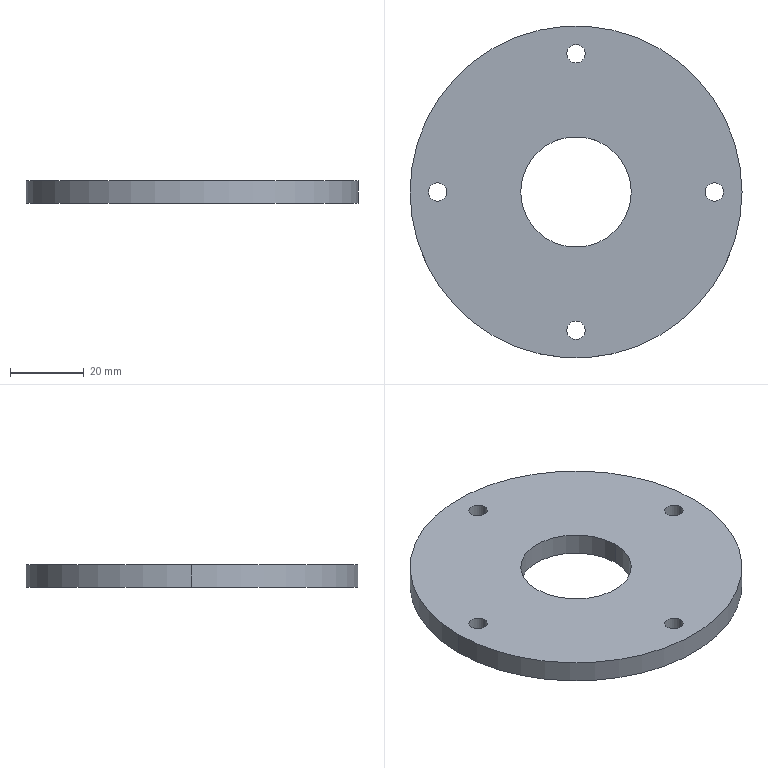Part | SolidWorks | features FlatPattern 1, HoleWzd 1, SMBaseFlange 1, SheetMetal 1 | 1 solid | 14 faces | box 90 x 90 x 6 mm | volume 33458 mm3 | cylinder 12 | plane 2 | commonest cylinder face diameters 5 x8 30 x2 90 x2
STEP:
#1=CARTESIAN_POINT('',(-2.5,37.5,-6.));
#2=VERTEX_POINT('',#1);
#3=CARTESIAN_POINT('',(2.5,37.5,-6.));
#4=VERTEX_POINT('',#3);
#5=CARTESIAN_POINT('',(0.,37.5,-6.));
#6=DIRECTION('',(0.,0.,1.));
#7=DIRECTION('',(1.,0.,0.));
#8=AXIS2_PLACEMENT_3D('',#5,#6,#7);
#9=CIRCLE('',#8,2.5);
#10=EDGE_CURVE('',#2,#4,#9,.T.);
#11=ORIENTED_EDGE('',*,*,#10,.F.);
#12=CARTESIAN_POINT('',(-2.5,37.5,0.));
#13=VERTEX_POINT('',#12);
#14=CARTESIAN_POINT('',(-2.5,37.5,0.));
#15=DIRECTION('',(0.,0.,1.));
#16=VECTOR('',#15,1000.);
#17=LINE('',#14,#16);
#18=EDGE_CURVE('',#2,#13,#17,.T.);
#19=ORIENTED_EDGE('',*,*,#18,.T.);
#20=CARTESIAN_POINT('',(2.5,37.5,0.));
#21=VERTEX_POINT('',#20);
#22=CARTESIAN_POINT('',(0.,37.5,0.));
#23=DIRECTION('',(0.,0.,1.));
#24=DIRECTION('',(1.,0.,0.));
#25=AXIS2_PLACEMENT_3D('',#22,#23,#24);
#26=CIRCLE('',#25,2.5);
#27=EDGE_CURVE('',#13,#21,#26,.T.);
#28=ORIENTED_EDGE('',*,*,#27,.T.);
#29=CARTESIAN_POINT('',(2.5,37.5,0.));
#30=DIRECTION('',(0.,0.,1.));
#31=VECTOR('',#30,1000.);
#32=LINE('',#29,#31);
#33=EDGE_CURVE('',#4,#21,#32,.T.);
#34=ORIENTED_EDGE('',*,*,#33,.F.);
#35=EDGE_LOOP('',(#11,#19,#28,#34));
#36=FACE_OUTER_BOUND('',#35,.T.);
#37=CARTESIAN_POINT('',(0.,37.5,0.));
#38=DIRECTION('',(0.,0.,1.));
#39=DIRECTION('',(1.,0.,0.));
#40=AXIS2_PLACEMENT_3D('',#37,#38,#39);
#41=CYLINDRICAL_SURFACE('',#40,2.5);
#42=ADVANCED_FACE('',(#36),#41,.F.);
#43=CARTESIAN_POINT('',(35.,0.,-6.));
#44=VERTEX_POINT('',#43);
#45=CARTESIAN_POINT('',(40.,0.,-6.));
#46=VERTEX_POINT('',#45);
#47=CARTESIAN_POINT('',(37.5,0.,-6.));
#48=DIRECTION('',(0.,0.,1.));
#49=DIRECTION('',(1.,0.,0.));
#50=AXIS2_PLACEMENT_3D('',#47,#48,#49);
#51=CIRCLE('',#50,2.5);
#52=EDGE_CURVE('',#44,#46,#51,.T.);
#53=ORIENTED_EDGE('',*,*,#52,.F.);
#54=CARTESIAN_POINT('',(35.,0.,0.));
#55=VERTEX_POINT('',#54);
#56=CARTESIAN_POINT('',(35.,0.,0.));
#57=DIRECTION('',(0.,0.,1.));
#58=VECTOR('',#57,1000.);
#59=LINE('',#56,#58);
#60=EDGE_CURVE('',#44,#55,#59,.T.);
#61=ORIENTED_EDGE('',*,*,#60,.T.);
#62=CARTESIAN_POINT('',(40.,0.,0.));
#63=VERTEX_POINT('',#62);
#64=CARTESIAN_POINT('',(37.5,0.,0.));
#65=DIRECTION('',(0.,0.,1.));
#66=DIRECTION('',(1.,0.,0.));
#67=AXIS2_PLACEMENT_3D('',#64,#65,#66);
#68=CIRCLE('',#67,2.5);
#69=EDGE_CURVE('',#55,#63,#68,.T.);
#70=ORIENTED_EDGE('',*,*,#69,.T.);
#71=CARTESIAN_POINT('',(40.,0.,0.));
#72=DIRECTION('',(0.,0.,1.));
#73=VECTOR('',#72,1000.);
#74=LINE('',#71,#73);
#75=EDGE_CURVE('',#46,#63,#74,.T.);
#76=ORIENTED_EDGE('',*,*,#75,.F.);
#77=EDGE_LOOP('',(#53,#61,#70,#76));
#78=FACE_OUTER_BOUND('',#77,.T.);
#79=CARTESIAN_POINT('',(37.5,0.,0.));
#80=DIRECTION('',(0.,0.,1.));
#81=DIRECTION('',(1.,0.,0.));
#82=AXIS2_PLACEMENT_3D('',#79,#80,#81);
#83=CYLINDRICAL_SURFACE('',#82,2.5);
#84=ADVANCED_FACE('',(#78),#83,.F.);
#85=CARTESIAN_POINT('',(-2.5,-37.5,-6.));
#86=VERTEX_POINT('',#85);
#87=CARTESIAN_POINT('',(2.5,-37.5,-6.));
#88=VERTEX_POINT('',#87);
#89=CARTESIAN_POINT('',(0.,-37.5,-6.));
#90=DIRECTION('',(0.,0.,1.));
#91=DIRECTION('',(1.,0.,0.));
#92=AXIS2_PLACEMENT_3D('',#89,#90,#91);
#93=CIRCLE('',#92,2.5);
#94=EDGE_CURVE('',#86,#88,#93,.T.);
#95=ORIENTED_EDGE('',*,*,#94,.F.);
#96=CARTESIAN_POINT('',(-2.5,-37.5,0.));
#97=VERTEX_POINT('',#96);
#98=CARTESIAN_POINT('',(-2.5,-37.5,0.));
#99=DIRECTION('',(0.,0.,1.));
#100=VECTOR('',#99,1000.);
#101=LINE('',#98,#100);
#102=EDGE_CURVE('',#86,#97,#101,.T.);
#103=ORIENTED_EDGE('',*,*,#102,.T.);
#104=CARTESIAN_POINT('',(2.5,-37.5,0.));
#105=VERTEX_POINT('',#104);
#106=CARTESIAN_POINT('',(0.,-37.5,0.));
#107=DIRECTION('',(0.,0.,1.));
#108=DIRECTION('',(1.,0.,0.));
#109=AXIS2_PLACEMENT_3D('',#106,#107,#108);
#110=CIRCLE('',#109,2.5);
#111=EDGE_CURVE('',#97,#105,#110,.T.);
#112=ORIENTED_EDGE('',*,*,#111,.T.);
#113=CARTESIAN_POINT('',(2.5,-37.5,0.));
#114=DIRECTION('',(0.,0.,1.));
#115=VECTOR('',#114,1000.);
#116=LINE('',#113,#115);
#117=EDGE_CURVE('',#88,#105,#116,.T.);
#118=ORIENTED_EDGE('',*,*,#117,.F.);
#119=EDGE_LOOP('',(#95,#103,#112,#118));
#120=FACE_OUTER_BOUND('',#119,.T.);
#121=CARTESIAN_POINT('',(0.,-37.5,0.));
#122=DIRECTION('',(0.,0.,1.));
#123=DIRECTION('',(1.,0.,0.));
#124=AXIS2_PLACEMENT_3D('',#121,#122,#123);
#125=CYLINDRICAL_SURFACE('',#124,2.5);
#126=ADVANCED_FACE('',(#120),#125,.F.);
#127=CARTESIAN_POINT('',(-40.,0.,-6.));
#128=VERTEX_POINT('',#127);
#129=CARTESIAN_POINT('',(-35.,0.,-6.));
#130=VERTEX_POINT('',#129);
#131=CARTESIAN_POINT('',(-37.5,0.,-6.));
#132=DIRECTION('',(0.,0.,1.));
#133=DIRECTION('',(1.,0.,0.));
#134=AXIS2_PLACEMENT_3D('',#131,#132,#133);
#135=CIRCLE('',#134,2.5);
#136=EDGE_CURVE('',#128,#130,#135,.T.);
#137=ORIENTED_EDGE('',*,*,#136,.F.);
#138=CARTESIAN_POINT('',(-40.,0.,0.));
#139=VERTEX_POINT('',#138);
#140=CARTESIAN_POINT('',(-40.,0.,0.));
#141=DIRECTION('',(0.,0.,1.));
#142=VECTOR('',#141,1000.);
#143=LINE('',#140,#142);
#144=EDGE_CURVE('',#128,#139,#143,.T.);
#145=ORIENTED_EDGE('',*,*,#144,.T.);
#146=CARTESIAN_POINT('',(-35.,0.,0.));
#147=VERTEX_POINT('',#146);
#148=CARTESIAN_POINT('',(-37.5,0.,0.));
#149=DIRECTION('',(0.,0.,1.));
#150=DIRECTION('',(1.,0.,0.));
#151=AXIS2_PLACEMENT_3D('',#148,#149,#150);
#152=CIRCLE('',#151,2.5);
#153=EDGE_CURVE('',#139,#147,#152,.T.);
#154=ORIENTED_EDGE('',*,*,#153,.T.);
#155=CARTESIAN_POINT('',(-35.,0.,0.));
#156=DIRECTION('',(0.,0.,1.));
#157=VECTOR('',#156,1000.);
#158=LINE('',#155,#157);
#159=EDGE_CURVE('',#130,#147,#158,.T.);
#160=ORIENTED_EDGE('',*,*,#159,.F.);
#161=EDGE_LOOP('',(#137,#145,#154,#160));
#162=FACE_OUTER_BOUND('',#161,.T.);
#163=CARTESIAN_POINT('',(-37.5,0.,0.));
#164=DIRECTION('',(0.,0.,1.));
#165=DIRECTION('',(1.,0.,0.));
#166=AXIS2_PLACEMENT_3D('',#163,#164,#165);
#167=CYLINDRICAL_SURFACE('',#166,2.5);
#168=ADVANCED_FACE('',(#162),#167,.F.);
#169=CARTESIAN_POINT('',(-15.,0.,-6.));
#170=VERTEX_POINT('',#169);
#171=CARTESIAN_POINT('',(15.,0.,-6.));
#172=VERTEX_POINT('',#171);
#173=CARTESIAN_POINT('',(0.,0.,-6.));
#174=DIRECTION('',(0.,0.,1.));
#175=DIRECTION('',(1.,0.,0.));
#176=AXIS2_PLACEMENT_3D('',#173,#174,#175);
#177=CIRCLE('',#176,15.);
#178=EDGE_CURVE('',#170,#172,#177,.T.);
#179=ORIENTED_EDGE('',*,*,#178,.F.);
#180=CARTESIAN_POINT('',(-15.,0.,0.));
#181=VERTEX_POINT('',#180);
#182=CARTESIAN_POINT('',(-15.,0.,-6.));
#183=DIRECTION('',(0.,0.,1.));
#184=VECTOR('',#183,1000.);
#185=LINE('',#182,#184);
#186=EDGE_CURVE('',#170,#181,#185,.T.);
#187=ORIENTED_EDGE('',*,*,#186,.T.);
#188=CARTESIAN_POINT('',(15.,0.,0.));
#189=VERTEX_POINT('',#188);
#190=CARTESIAN_POINT('',(0.,0.,0.));
#191=DIRECTION('',(0.,0.,1.));
#192=DIRECTION('',(1.,0.,0.));
#193=AXIS2_PLACEMENT_3D('',#190,#191,#192);
#194=CIRCLE('',#193,15.);
#195=EDGE_CURVE('',#181,#189,#194,.T.);
#196=ORIENTED_EDGE('',*,*,#195,.T.);
#197=CARTESIAN_POINT('',(15.,0.,-6.));
#198=DIRECTION('',(0.,0.,1.));
#199=VECTOR('',#198,1000.);
#200=LINE('',#197,#199);
#201=EDGE_CURVE('',#172,#189,#200,.T.);
#202=ORIENTED_EDGE('',*,*,#201,.F.);
#203=EDGE_LOOP('',(#179,#187,#196,#202));
#204=FACE_OUTER_BOUND('',#203,.T.);
#205=CARTESIAN_POINT('',(0.,0.,-6.));
#206=DIRECTION('',(0.,0.,1.));
#207=DIRECTION('',(1.,0.,0.));
#208=AXIS2_PLACEMENT_3D('',#205,#206,#207);
#209=CYLINDRICAL_SURFACE('',#208,15.);
#210=ADVANCED_FACE('',(#204),#209,.F.);
#211=CARTESIAN_POINT('',(45.,0.,-6.));
#212=VERTEX_POINT('',#211);
#213=CARTESIAN_POINT('',(-45.,0.,-6.));
#214=VERTEX_POINT('',#213);
#215=CARTESIAN_POINT('',(0.,0.,-6.));
#216=DIRECTION('',(0.,0.,1.));
#217=DIRECTION('',(1.,0.,0.));
#218=AXIS2_PLACEMENT_3D('',#215,#216,#217);
#219=CIRCLE('',#218,45.);
#220=EDGE_CURVE('',#212,#214,#219,.T.);
#221=ORIENTED_EDGE('',*,*,#220,.T.);
#222=CARTESIAN_POINT('',(-45.,0.,0.));
#223=VERTEX_POINT('',#222);
#224=CARTESIAN_POINT('',(-45.,0.,-6.));
#225=DIRECTION('',(0.,0.,1.));
#226=VECTOR('',#225,1000.);
#227=LINE('',#224,#226);
#228=EDGE_CURVE('',#214,#223,#227,.T.);
#229=ORIENTED_EDGE('',*,*,#228,.T.);
#230=CARTESIAN_POINT('',(45.,0.,0.));
#231=VERTEX_POINT('',#230);
#232=CARTESIAN_POINT('',(0.,0.,0.));
#233=DIRECTION('',(0.,0.,1.));
#234=DIRECTION('',(1.,0.,0.));
#235=AXIS2_PLACEMENT_3D('',#232,#233,#234);
#236=CIRCLE('',#235,45.);
#237=EDGE_CURVE('',#231,#223,#236,.T.);
#238=ORIENTED_EDGE('',*,*,#237,.F.);
#239=CARTESIAN_POINT('',(45.,0.,-6.));
#240=DIRECTION('',(0.,0.,1.));
#241=VECTOR('',#240,1000.);
#242=LINE('',#239,#241);
#243=EDGE_CURVE('',#212,#231,#242,.T.);
#244=ORIENTED_EDGE('',*,*,#243,.F.);
#245=EDGE_LOOP('',(#221,#229,#238,#244));
#246=FACE_OUTER_BOUND('',#245,.T.);
#247=CARTESIAN_POINT('',(0.,0.,-6.));
#248=DIRECTION('',(0.,0.,1.));
#249=DIRECTION('',(1.,0.,0.));
#250=AXIS2_PLACEMENT_3D('',#247,#248,#249);
#251=CYLINDRICAL_SURFACE('',#250,45.);
#252=ADVANCED_FACE('',(#246),#251,.T.);
#253=ORIENTED_EDGE('',*,*,#228,.F.);
#254=CARTESIAN_POINT('',(0.,0.,-6.));
#255=DIRECTION('',(0.,0.,1.));
#256=DIRECTION('',(1.,0.,0.));
#257=AXIS2_PLACEMENT_3D('',#254,#255,#256);
#258=CIRCLE('',#257,45.);
#259=EDGE_CURVE('',#214,#212,#258,.T.);
#260=ORIENTED_EDGE('',*,*,#259,.T.);
#261=ORIENTED_EDGE('',*,*,#243,.T.);
#262=CARTESIAN_POINT('',(0.,0.,0.));
#263=DIRECTION('',(0.,0.,1.));
#264=DIRECTION('',(1.,0.,0.));
#265=AXIS2_PLACEMENT_3D('',#262,#263,#264);
#266=CIRCLE('',#265,45.);
#267=EDGE_CURVE('',#223,#231,#266,.T.);
#268=ORIENTED_EDGE('',*,*,#267,.F.);
#269=EDGE_LOOP('',(#253,#260,#261,#268));
#270=FACE_OUTER_BOUND('',#269,.T.);
#271=CARTESIAN_POINT('',(0.,0.,-6.));
#272=DIRECTION('',(0.,0.,1.));
#273=DIRECTION('',(1.,0.,0.));
#274=AXIS2_PLACEMENT_3D('',#271,#272,#273);
#275=CYLINDRICAL_SURFACE('',#274,45.);
#276=ADVANCED_FACE('',(#270),#275,.T.);
#277=CARTESIAN_POINT('',(0.,37.5,-6.));
#278=DIRECTION('',(0.,0.,1.));
#279=DIRECTION('',(1.,0.,0.));
#280=AXIS2_PLACEMENT_3D('',#277,#278,#279);
#281=CIRCLE('',#280,2.5);
#282=EDGE_CURVE('',#4,#2,#281,.T.);
#283=ORIENTED_EDGE('',*,*,#282,.T.);
#284=ORIENTED_EDGE('',*,*,#10,.T.);
#285=EDGE_LOOP('',(#283,#284));
#286=FACE_BOUND('',#285,.T.);
#287=CARTESIAN_POINT('',(37.5,0.,-6.));
#288=DIRECTION('',(0.,0.,1.));
#289=DIRECTION('',(1.,0.,0.));
#290=AXIS2_PLACEMENT_3D('',#287,#288,#289);
#291=CIRCLE('',#290,2.5);
#292=EDGE_CURVE('',#46,#44,#291,.T.);
#293=ORIENTED_EDGE('',*,*,#292,.T.);
#294=ORIENTED_EDGE('',*,*,#52,.T.);
#295=EDGE_LOOP('',(#293,#294));
#296=FACE_BOUND('',#295,.T.);
#297=CARTESIAN_POINT('',(0.,-37.5,-6.));
#298=DIRECTION('',(0.,0.,1.));
#299=DIRECTION('',(1.,0.,0.));
#300=AXIS2_PLACEMENT_3D('',#297,#298,#299);
#301=CIRCLE('',#300,2.5);
#302=EDGE_CURVE('',#88,#86,#301,.T.);
#303=ORIENTED_EDGE('',*,*,#302,.T.);
#304=ORIENTED_EDGE('',*,*,#94,.T.);
#305=EDGE_LOOP('',(#303,#304));
#306=FACE_BOUND('',#305,.T.);
#307=CARTESIAN_POINT('',(-37.5,0.,-6.));
#308=DIRECTION('',(0.,0.,1.));
#309=DIRECTION('',(1.,0.,0.));
#310=AXIS2_PLACEMENT_3D('',#307,#308,#309);
#311=CIRCLE('',#310,2.5);
#312=EDGE_CURVE('',#130,#128,#311,.T.);
#313=ORIENTED_EDGE('',*,*,#312,.T.);
#314=ORIENTED_EDGE('',*,*,#136,.T.);
#315=EDGE_LOOP('',(#313,#314));
#316=FACE_BOUND('',#315,.T.);
#317=CARTESIAN_POINT('',(0.,0.,-6.));
#318=DIRECTION('',(0.,0.,1.));
#319=DIRECTION('',(1.,0.,0.));
#320=AXIS2_PLACEMENT_3D('',#317,#318,#319);
#321=CIRCLE('',#320,15.);
#322=EDGE_CURVE('',#172,#170,#321,.T.);
#323=ORIENTED_EDGE('',*,*,#322,.T.);
#324=ORIENTED_EDGE('',*,*,#178,.T.);
#325=EDGE_LOOP('',(#323,#324));
#326=FACE_BOUND('',#325,.T.);
#327=ORIENTED_EDGE('',*,*,#220,.F.);
#328=ORIENTED_EDGE('',*,*,#259,.F.);
#329=EDGE_LOOP('',(#327,#328));
#330=FACE_OUTER_BOUND('',#329,.T.);
#331=CARTESIAN_POINT('',(0.,0.,-6.));
#332=DIRECTION('',(0.,0.,1.));
#333=DIRECTION('',(1.,0.,0.));
#334=AXIS2_PLACEMENT_3D('',#331,#332,#333);
#335=PLANE('',#334);
#336=ADVANCED_FACE('',(#286,#296,#306,#316,#326,#330),#335,.F.);
#337=CARTESIAN_POINT('',(0.,37.5,0.));
#338=DIRECTION('',(0.,0.,1.));
#339=DIRECTION('',(1.,0.,0.));
#340=AXIS2_PLACEMENT_3D('',#337,#338,#339);
#341=CIRCLE('',#340,2.5);
#342=EDGE_CURVE('',#21,#13,#341,.T.);
#343=ORIENTED_EDGE('',*,*,#342,.F.);
#344=ORIENTED_EDGE('',*,*,#27,.F.);
#345=EDGE_LOOP('',(#343,#344));
#346=FACE_BOUND('',#345,.T.);
#347=CARTESIAN_POINT('',(37.5,0.,0.));
#348=DIRECTION('',(0.,0.,1.));
#349=DIRECTION('',(1.,0.,0.));
#350=AXIS2_PLACEMENT_3D('',#347,#348,#349);
#351=CIRCLE('',#350,2.5);
#352=EDGE_CURVE('',#63,#55,#351,.T.);
#353=ORIENTED_EDGE('',*,*,#352,.F.);
#354=ORIENTED_EDGE('',*,*,#69,.F.);
#355=EDGE_LOOP('',(#353,#354));
#356=FACE_BOUND('',#355,.T.);
#357=CARTESIAN_POINT('',(0.,-37.5,0.));
#358=DIRECTION('',(0.,0.,1.));
#359=DIRECTION('',(1.,0.,0.));
#360=AXIS2_PLACEMENT_3D('',#357,#358,#359);
#361=CIRCLE('',#360,2.5);
#362=EDGE_CURVE('',#105,#97,#361,.T.);
#363=ORIENTED_EDGE('',*,*,#362,.F.);
#364=ORIENTED_EDGE('',*,*,#111,.F.);
#365=EDGE_LOOP('',(#363,#364));
#366=FACE_BOUND('',#365,.T.);
#367=CARTESIAN_POINT('',(-37.5,0.,0.));
#368=DIRECTION('',(0.,0.,1.));
#369=DIRECTION('',(1.,0.,0.));
#370=AXIS2_PLACEMENT_3D('',#367,#368,#369);
#371=CIRCLE('',#370,2.5);
#372=EDGE_CURVE('',#147,#139,#371,.T.);
#373=ORIENTED_EDGE('',*,*,#372,.F.);
#374=ORIENTED_EDGE('',*,*,#153,.F.);
#375=EDGE_LOOP('',(#373,#374));
#376=FACE_BOUND('',#375,.T.);
#377=CARTESIAN_POINT('',(0.,0.,0.));
#378=DIRECTION('',(0.,0.,1.));
#379=DIRECTION('',(1.,0.,0.));
#380=AXIS2_PLACEMENT_3D('',#377,#378,#379);
#381=CIRCLE('',#380,15.);
#382=EDGE_CURVE('',#189,#181,#381,.T.);
#383=ORIENTED_EDGE('',*,*,#382,.F.);
#384=ORIENTED_EDGE('',*,*,#195,.F.);
#385=EDGE_LOOP('',(#383,#384));
#386=FACE_BOUND('',#385,.T.);
#387=ORIENTED_EDGE('',*,*,#237,.T.);
#388=ORIENTED_EDGE('',*,*,#267,.T.);
#389=EDGE_LOOP('',(#387,#388));
#390=FACE_OUTER_BOUND('',#389,.T.);
#391=CARTESIAN_POINT('',(0.,0.,0.));
#392=DIRECTION('',(0.,0.,1.));
#393=DIRECTION('',(1.,0.,0.));
#394=AXIS2_PLACEMENT_3D('',#391,#392,#393);
#395=PLANE('',#394);
#396=ADVANCED_FACE('',(#346,#356,#366,#376,#386,#390),#395,.T.);
#397=ORIENTED_EDGE('',*,*,#186,.F.);
#398=ORIENTED_EDGE('',*,*,#322,.F.);
#399=ORIENTED_EDGE('',*,*,#201,.T.);
#400=ORIENTED_EDGE('',*,*,#382,.T.);
#401=EDGE_LOOP('',(#397,#398,#399,#400));
#402=FACE_OUTER_BOUND('',#401,.T.);
#403=CARTESIAN_POINT('',(0.,0.,-6.));
#404=DIRECTION('',(0.,0.,1.));
#405=DIRECTION('',(1.,0.,0.));
#406=AXIS2_PLACEMENT_3D('',#403,#404,#405);
#407=CYLINDRICAL_SURFACE('',#406,15.);
#408=ADVANCED_FACE('',(#402),#407,.F.);
#409=ORIENTED_EDGE('',*,*,#144,.F.);
#410=ORIENTED_EDGE('',*,*,#312,.F.);
#411=ORIENTED_EDGE('',*,*,#159,.T.);
#412=ORIENTED_EDGE('',*,*,#372,.T.);
#413=EDGE_LOOP('',(#409,#410,#411,#412));
#414=FACE_OUTER_BOUND('',#413,.T.);
#415=CARTESIAN_POINT('',(-37.5,0.,0.));
#416=DIRECTION('',(0.,0.,1.));
#417=DIRECTION('',(1.,0.,0.));
#418=AXIS2_PLACEMENT_3D('',#415,#416,#417);
#419=CYLINDRICAL_SURFACE('',#418,2.5);
#420=ADVANCED_FACE('',(#414),#419,.F.);
#421=ORIENTED_EDGE('',*,*,#102,.F.);
#422=ORIENTED_EDGE('',*,*,#302,.F.);
#423=ORIENTED_EDGE('',*,*,#117,.T.);
#424=ORIENTED_EDGE('',*,*,#362,.T.);
#425=EDGE_LOOP('',(#421,#422,#423,#424));
#426=FACE_OUTER_BOUND('',#425,.T.);
#427=CARTESIAN_POINT('',(0.,-37.5,0.));
#428=DIRECTION('',(0.,0.,1.));
#429=DIRECTION('',(1.,0.,0.));
#430=AXIS2_PLACEMENT_3D('',#427,#428,#429);
#431=CYLINDRICAL_SURFACE('',#430,2.5);
#432=ADVANCED_FACE('',(#426),#431,.F.);
#433=ORIENTED_EDGE('',*,*,#60,.F.);
#434=ORIENTED_EDGE('',*,*,#292,.F.);
#435=ORIENTED_EDGE('',*,*,#75,.T.);
#436=ORIENTED_EDGE('',*,*,#352,.T.);
#437=EDGE_LOOP('',(#433,#434,#435,#436));
#438=FACE_OUTER_BOUND('',#437,.T.);
#439=CARTESIAN_POINT('',(37.5,0.,0.));
#440=DIRECTION('',(0.,0.,1.));
#441=DIRECTION('',(1.,0.,0.));
#442=AXIS2_PLACEMENT_3D('',#439,#440,#441);
#443=CYLINDRICAL_SURFACE('',#442,2.5);
#444=ADVANCED_FACE('',(#438),#443,.F.);
#445=ORIENTED_EDGE('',*,*,#18,.F.);
#446=ORIENTED_EDGE('',*,*,#282,.F.);
#447=ORIENTED_EDGE('',*,*,#33,.T.);
#448=ORIENTED_EDGE('',*,*,#342,.T.);
#449=EDGE_LOOP('',(#445,#446,#447,#448));
#450=FACE_OUTER_BOUND('',#449,.T.);
#451=CARTESIAN_POINT('',(0.,37.5,0.));
#452=DIRECTION('',(0.,0.,1.));
#453=DIRECTION('',(1.,0.,0.));
#454=AXIS2_PLACEMENT_3D('',#451,#452,#453);
#455=CYLINDRICAL_SURFACE('',#454,2.5);
#456=ADVANCED_FACE('',(#450),#455,.F.);
#457=CLOSED_SHELL('',(#42,#84,#126,#168,#210,#252,#276,#336,#396,#408,#420,#432,#444,#456));
#458=MANIFOLD_SOLID_BREP('',#457);
#459=CARTESIAN_POINT('',(0.,0.,0.));
#460=DIRECTION('',(0.,0.,1.));
#461=DIRECTION('',(1.,0.,0.));
#462=AXIS2_PLACEMENT_3D('',#459,#460,#461);
#463=(LENGTH_UNIT()NAMED_UNIT(*)SI_UNIT(.MILLI.,.METRE.));
#464=UNCERTAINTY_MEASURE_WITH_UNIT(LENGTH_MEASURE(0.00001),#463,'','');
#465=(NAMED_UNIT(*)PLANE_ANGLE_UNIT()SI_UNIT($,.RADIAN.));
#466=(NAMED_UNIT(*)SI_UNIT($,.STERADIAN.)SOLID_ANGLE_UNIT());
#467=(GEOMETRIC_REPRESENTATION_CONTEXT(3)GLOBAL_UNCERTAINTY_ASSIGNED_CONTEXT((#464))GLOBAL_UNIT_ASSIGNED_CONTEXT((#463,#465,#466))REPRESENTATION_CONTEXT('',''));
#468=ADVANCED_BREP_SHAPE_REPRESENTATION('',(#458,#462),#467);